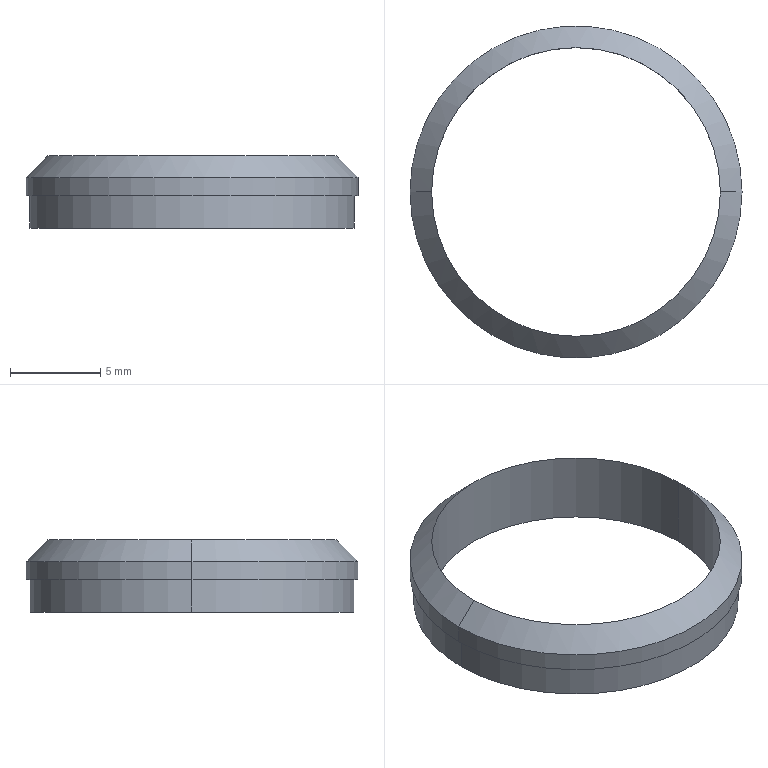Part | SolidWorks | features Revolution 1 | 1 solid | 10 faces | box 18.4 x 18.4 x 4 mm | volume 198.976 mm3 | cylinder 6 | cone 2 | plane 2 | commonest cylinder face diameters 16 x2 18 x2 18.4 x2
STEP:
#1=CARTESIAN_POINT('',(9.,0.,-4.));
#2=VERTEX_POINT('',#1);
#3=CARTESIAN_POINT('',(-9.,0.,-4.));
#4=VERTEX_POINT('',#3);
#5=CARTESIAN_POINT('',(0.,0.,-4.));
#6=DIRECTION('',(0.,0.,1.));
#7=DIRECTION('',(1.,0.,0.));
#8=AXIS2_PLACEMENT_3D('',#5,#6,#7);
#9=CIRCLE('',#8,9.);
#10=EDGE_CURVE('',#2,#4,#9,.T.);
#11=ORIENTED_EDGE('',*,*,#10,.T.);
#12=CARTESIAN_POINT('',(-9.,0.,-2.2));
#13=VERTEX_POINT('',#12);
#14=CARTESIAN_POINT('',(-9.,0.,-4.));
#15=DIRECTION('',(0.,0.,1.));
#16=VECTOR('',#15,1000.);
#17=LINE('',#14,#16);
#18=EDGE_CURVE('',#4,#13,#17,.T.);
#19=ORIENTED_EDGE('',*,*,#18,.T.);
#20=CARTESIAN_POINT('',(9.,0.,-2.2));
#21=VERTEX_POINT('',#20);
#22=CARTESIAN_POINT('',(0.,0.,-2.2));
#23=DIRECTION('',(0.,0.,1.));
#24=DIRECTION('',(1.,0.,0.));
#25=AXIS2_PLACEMENT_3D('',#22,#23,#24);
#26=CIRCLE('',#25,9.);
#27=EDGE_CURVE('',#21,#13,#26,.T.);
#28=ORIENTED_EDGE('',*,*,#27,.F.);
#29=CARTESIAN_POINT('',(9.,0.,-4.));
#30=DIRECTION('',(0.,0.,1.));
#31=VECTOR('',#30,1000.);
#32=LINE('',#29,#31);
#33=EDGE_CURVE('',#2,#21,#32,.T.);
#34=ORIENTED_EDGE('',*,*,#33,.F.);
#35=EDGE_LOOP('',(#11,#19,#28,#34));
#36=FACE_OUTER_BOUND('',#35,.T.);
#37=CARTESIAN_POINT('',(0.,0.,-4.));
#38=DIRECTION('',(0.,0.,1.));
#39=DIRECTION('',(1.,0.,0.));
#40=AXIS2_PLACEMENT_3D('',#37,#38,#39);
#41=CYLINDRICAL_SURFACE('',#40,9.);
#42=ADVANCED_FACE('',(#36),#41,.T.);
#43=CARTESIAN_POINT('',(9.2,0.,-2.2));
#44=VERTEX_POINT('',#43);
#45=CARTESIAN_POINT('',(-9.2,0.,-2.2));
#46=VERTEX_POINT('',#45);
#47=CARTESIAN_POINT('',(0.,0.,-2.2));
#48=DIRECTION('',(0.,0.,1.));
#49=DIRECTION('',(1.,0.,0.));
#50=AXIS2_PLACEMENT_3D('',#47,#48,#49);
#51=CIRCLE('',#50,9.2);
#52=EDGE_CURVE('',#44,#46,#51,.T.);
#53=ORIENTED_EDGE('',*,*,#52,.T.);
#54=CARTESIAN_POINT('',(-9.2,0.,-1.2));
#55=VERTEX_POINT('',#54);
#56=CARTESIAN_POINT('',(-9.2,0.,-4.));
#57=DIRECTION('',(0.,0.,1.));
#58=VECTOR('',#57,1000.);
#59=LINE('',#56,#58);
#60=EDGE_CURVE('',#46,#55,#59,.T.);
#61=ORIENTED_EDGE('',*,*,#60,.T.);
#62=CARTESIAN_POINT('',(9.2,0.,-1.2));
#63=VERTEX_POINT('',#62);
#64=CARTESIAN_POINT('',(0.,0.,-1.2));
#65=DIRECTION('',(0.,0.,1.));
#66=DIRECTION('',(1.,0.,0.));
#67=AXIS2_PLACEMENT_3D('',#64,#65,#66);
#68=CIRCLE('',#67,9.2);
#69=EDGE_CURVE('',#63,#55,#68,.T.);
#70=ORIENTED_EDGE('',*,*,#69,.F.);
#71=CARTESIAN_POINT('',(9.2,0.,-4.));
#72=DIRECTION('',(0.,0.,1.));
#73=VECTOR('',#72,1000.);
#74=LINE('',#71,#73);
#75=EDGE_CURVE('',#44,#63,#74,.T.);
#76=ORIENTED_EDGE('',*,*,#75,.F.);
#77=EDGE_LOOP('',(#53,#61,#70,#76));
#78=FACE_OUTER_BOUND('',#77,.T.);
#79=CARTESIAN_POINT('',(0.,0.,-4.));
#80=DIRECTION('',(0.,0.,1.));
#81=DIRECTION('',(1.,0.,0.));
#82=AXIS2_PLACEMENT_3D('',#79,#80,#81);
#83=CYLINDRICAL_SURFACE('',#82,9.2);
#84=ADVANCED_FACE('',(#78),#83,.T.);
#85=CARTESIAN_POINT('',(8.,0.,0.));
#86=VERTEX_POINT('',#85);
#87=CARTESIAN_POINT('',(-8.,0.,0.));
#88=VERTEX_POINT('',#87);
#89=CARTESIAN_POINT('',(0.,0.,0.));
#90=DIRECTION('',(0.,0.,1.));
#91=DIRECTION('',(1.,0.,0.));
#92=AXIS2_PLACEMENT_3D('',#89,#90,#91);
#93=CIRCLE('',#92,8.);
#94=EDGE_CURVE('',#86,#88,#93,.T.);
#95=ORIENTED_EDGE('',*,*,#94,.F.);
#96=CARTESIAN_POINT('',(8.,0.,0.));
#97=DIRECTION('',(0.7071,0.,-0.7071));
#98=VECTOR('',#97,1000.);
#99=LINE('',#96,#98);
#100=EDGE_CURVE('',#86,#63,#99,.T.);
#101=ORIENTED_EDGE('',*,*,#100,.T.);
#102=ORIENTED_EDGE('',*,*,#69,.T.);
#103=CARTESIAN_POINT('',(-8.,0.,0.));
#104=DIRECTION('',(-0.7071,0.,-0.7071));
#105=VECTOR('',#104,1000.);
#106=LINE('',#103,#105);
#107=EDGE_CURVE('',#88,#55,#106,.T.);
#108=ORIENTED_EDGE('',*,*,#107,.F.);
#109=EDGE_LOOP('',(#95,#101,#102,#108));
#110=FACE_OUTER_BOUND('',#109,.T.);
#111=CARTESIAN_POINT('',(0.,0.,0.));
#112=DIRECTION('',(0.,0.,-1.));
#113=DIRECTION('',(-1.,0.,0.));
#114=AXIS2_PLACEMENT_3D('',#111,#112,#113);
#115=CONICAL_SURFACE('',#114,8.,0.7854);
#116=ADVANCED_FACE('',(#110),#115,.T.);
#117=CARTESIAN_POINT('',(-8.,0.,-4.));
#118=VERTEX_POINT('',#117);
#119=CARTESIAN_POINT('',(8.,0.,-4.));
#120=VERTEX_POINT('',#119);
#121=CARTESIAN_POINT('',(0.,0.,-4.));
#122=DIRECTION('',(0.,0.,1.));
#123=DIRECTION('',(1.,0.,0.));
#124=AXIS2_PLACEMENT_3D('',#121,#122,#123);
#125=CIRCLE('',#124,8.);
#126=EDGE_CURVE('',#118,#120,#125,.T.);
#127=ORIENTED_EDGE('',*,*,#126,.F.);
#128=CARTESIAN_POINT('',(-8.,0.,-4.));
#129=DIRECTION('',(0.,0.,1.));
#130=VECTOR('',#129,1000.);
#131=LINE('',#128,#130);
#132=EDGE_CURVE('',#118,#88,#131,.T.);
#133=ORIENTED_EDGE('',*,*,#132,.T.);
#134=CARTESIAN_POINT('',(0.,0.,0.));
#135=DIRECTION('',(0.,0.,1.));
#136=DIRECTION('',(1.,0.,0.));
#137=AXIS2_PLACEMENT_3D('',#134,#135,#136);
#138=CIRCLE('',#137,8.);
#139=EDGE_CURVE('',#88,#86,#138,.T.);
#140=ORIENTED_EDGE('',*,*,#139,.T.);
#141=CARTESIAN_POINT('',(8.,0.,-4.));
#142=DIRECTION('',(0.,0.,1.));
#143=VECTOR('',#142,1000.);
#144=LINE('',#141,#143);
#145=EDGE_CURVE('',#120,#86,#144,.T.);
#146=ORIENTED_EDGE('',*,*,#145,.F.);
#147=EDGE_LOOP('',(#127,#133,#140,#146));
#148=FACE_OUTER_BOUND('',#147,.T.);
#149=CARTESIAN_POINT('',(0.,0.,-4.));
#150=DIRECTION('',(0.,0.,1.));
#151=DIRECTION('',(1.,0.,0.));
#152=AXIS2_PLACEMENT_3D('',#149,#150,#151);
#153=CYLINDRICAL_SURFACE('',#152,8.);
#154=ADVANCED_FACE('',(#148),#153,.F.);
#155=CARTESIAN_POINT('',(0.,0.,-4.));
#156=DIRECTION('',(0.,0.,1.));
#157=DIRECTION('',(1.,0.,0.));
#158=AXIS2_PLACEMENT_3D('',#155,#156,#157);
#159=CIRCLE('',#158,8.);
#160=EDGE_CURVE('',#120,#118,#159,.T.);
#161=ORIENTED_EDGE('',*,*,#160,.T.);
#162=ORIENTED_EDGE('',*,*,#126,.T.);
#163=EDGE_LOOP('',(#161,#162));
#164=FACE_BOUND('',#163,.T.);
#165=ORIENTED_EDGE('',*,*,#10,.F.);
#166=CARTESIAN_POINT('',(0.,0.,-4.));
#167=DIRECTION('',(0.,0.,1.));
#168=DIRECTION('',(1.,0.,0.));
#169=AXIS2_PLACEMENT_3D('',#166,#167,#168);
#170=CIRCLE('',#169,9.);
#171=EDGE_CURVE('',#4,#2,#170,.T.);
#172=ORIENTED_EDGE('',*,*,#171,.F.);
#173=EDGE_LOOP('',(#165,#172));
#174=FACE_OUTER_BOUND('',#173,.T.);
#175=CARTESIAN_POINT('',(9.,0.,-4.));
#176=DIRECTION('',(0.,0.,-1.));
#177=DIRECTION('',(-1.,0.,0.));
#178=AXIS2_PLACEMENT_3D('',#175,#176,#177);
#179=PLANE('',#178);
#180=ADVANCED_FACE('',(#164,#174),#179,.T.);
#181=ORIENTED_EDGE('',*,*,#132,.F.);
#182=ORIENTED_EDGE('',*,*,#160,.F.);
#183=ORIENTED_EDGE('',*,*,#145,.T.);
#184=ORIENTED_EDGE('',*,*,#94,.T.);
#185=EDGE_LOOP('',(#181,#182,#183,#184));
#186=FACE_OUTER_BOUND('',#185,.T.);
#187=CARTESIAN_POINT('',(0.,0.,-4.));
#188=DIRECTION('',(0.,0.,1.));
#189=DIRECTION('',(1.,0.,0.));
#190=AXIS2_PLACEMENT_3D('',#187,#188,#189);
#191=CYLINDRICAL_SURFACE('',#190,8.);
#192=ADVANCED_FACE('',(#186),#191,.F.);
#193=ORIENTED_EDGE('',*,*,#100,.F.);
#194=ORIENTED_EDGE('',*,*,#139,.F.);
#195=ORIENTED_EDGE('',*,*,#107,.T.);
#196=CARTESIAN_POINT('',(0.,0.,-1.2));
#197=DIRECTION('',(0.,0.,1.));
#198=DIRECTION('',(1.,0.,0.));
#199=AXIS2_PLACEMENT_3D('',#196,#197,#198);
#200=CIRCLE('',#199,9.2);
#201=EDGE_CURVE('',#55,#63,#200,.T.);
#202=ORIENTED_EDGE('',*,*,#201,.T.);
#203=EDGE_LOOP('',(#193,#194,#195,#202));
#204=FACE_OUTER_BOUND('',#203,.T.);
#205=CARTESIAN_POINT('',(0.,0.,0.));
#206=DIRECTION('',(0.,0.,-1.));
#207=DIRECTION('',(-1.,0.,0.));
#208=AXIS2_PLACEMENT_3D('',#205,#206,#207);
#209=CONICAL_SURFACE('',#208,8.,0.7854);
#210=ADVANCED_FACE('',(#204),#209,.T.);
#211=ORIENTED_EDGE('',*,*,#60,.F.);
#212=CARTESIAN_POINT('',(0.,0.,-2.2));
#213=DIRECTION('',(0.,0.,1.));
#214=DIRECTION('',(1.,0.,0.));
#215=AXIS2_PLACEMENT_3D('',#212,#213,#214);
#216=CIRCLE('',#215,9.2);
#217=EDGE_CURVE('',#46,#44,#216,.T.);
#218=ORIENTED_EDGE('',*,*,#217,.T.);
#219=ORIENTED_EDGE('',*,*,#75,.T.);
#220=ORIENTED_EDGE('',*,*,#201,.F.);
#221=EDGE_LOOP('',(#211,#218,#219,#220));
#222=FACE_OUTER_BOUND('',#221,.T.);
#223=CARTESIAN_POINT('',(0.,0.,-4.));
#224=DIRECTION('',(0.,0.,1.));
#225=DIRECTION('',(1.,0.,0.));
#226=AXIS2_PLACEMENT_3D('',#223,#224,#225);
#227=CYLINDRICAL_SURFACE('',#226,9.2);
#228=ADVANCED_FACE('',(#222),#227,.T.);
#229=ORIENTED_EDGE('',*,*,#27,.T.);
#230=CARTESIAN_POINT('',(0.,0.,-2.2));
#231=DIRECTION('',(0.,0.,1.));
#232=DIRECTION('',(1.,0.,0.));
#233=AXIS2_PLACEMENT_3D('',#230,#231,#232);
#234=CIRCLE('',#233,9.);
#235=EDGE_CURVE('',#13,#21,#234,.T.);
#236=ORIENTED_EDGE('',*,*,#235,.T.);
#237=EDGE_LOOP('',(#229,#236));
#238=FACE_BOUND('',#237,.T.);
#239=ORIENTED_EDGE('',*,*,#52,.F.);
#240=ORIENTED_EDGE('',*,*,#217,.F.);
#241=EDGE_LOOP('',(#239,#240));
#242=FACE_OUTER_BOUND('',#241,.T.);
#243=CARTESIAN_POINT('',(9.2,0.,-2.2));
#244=DIRECTION('',(0.,0.,-1.));
#245=DIRECTION('',(-1.,0.,0.));
#246=AXIS2_PLACEMENT_3D('',#243,#244,#245);
#247=PLANE('',#246);
#248=ADVANCED_FACE('',(#238,#242),#247,.T.);
#249=ORIENTED_EDGE('',*,*,#18,.F.);
#250=ORIENTED_EDGE('',*,*,#171,.T.);
#251=ORIENTED_EDGE('',*,*,#33,.T.);
#252=ORIENTED_EDGE('',*,*,#235,.F.);
#253=EDGE_LOOP('',(#249,#250,#251,#252));
#254=FACE_OUTER_BOUND('',#253,.T.);
#255=CARTESIAN_POINT('',(0.,0.,-4.));
#256=DIRECTION('',(0.,0.,1.));
#257=DIRECTION('',(1.,0.,0.));
#258=AXIS2_PLACEMENT_3D('',#255,#256,#257);
#259=CYLINDRICAL_SURFACE('',#258,9.);
#260=ADVANCED_FACE('',(#254),#259,.T.);
#261=CLOSED_SHELL('',(#42,#84,#116,#154,#180,#192,#210,#228,#248,#260));
#262=MANIFOLD_SOLID_BREP('',#261);
#263=CARTESIAN_POINT('',(0.,0.,0.));
#264=DIRECTION('',(0.,0.,1.));
#265=DIRECTION('',(1.,0.,0.));
#266=AXIS2_PLACEMENT_3D('',#263,#264,#265);
#267=(LENGTH_UNIT()NAMED_UNIT(*)SI_UNIT(.MILLI.,.METRE.));
#268=UNCERTAINTY_MEASURE_WITH_UNIT(LENGTH_MEASURE(0.00001),#267,'','');
#269=(NAMED_UNIT(*)PLANE_ANGLE_UNIT()SI_UNIT($,.RADIAN.));
#270=(NAMED_UNIT(*)SI_UNIT($,.STERADIAN.)SOLID_ANGLE_UNIT());
#271=(GEOMETRIC_REPRESENTATION_CONTEXT(3)GLOBAL_UNCERTAINTY_ASSIGNED_CONTEXT((#268))GLOBAL_UNIT_ASSIGNED_CONTEXT((#267,#269,#270))REPRESENTATION_CONTEXT('',''));
#272=ADVANCED_BREP_SHAPE_REPRESENTATION('',(#262,#266),#271);